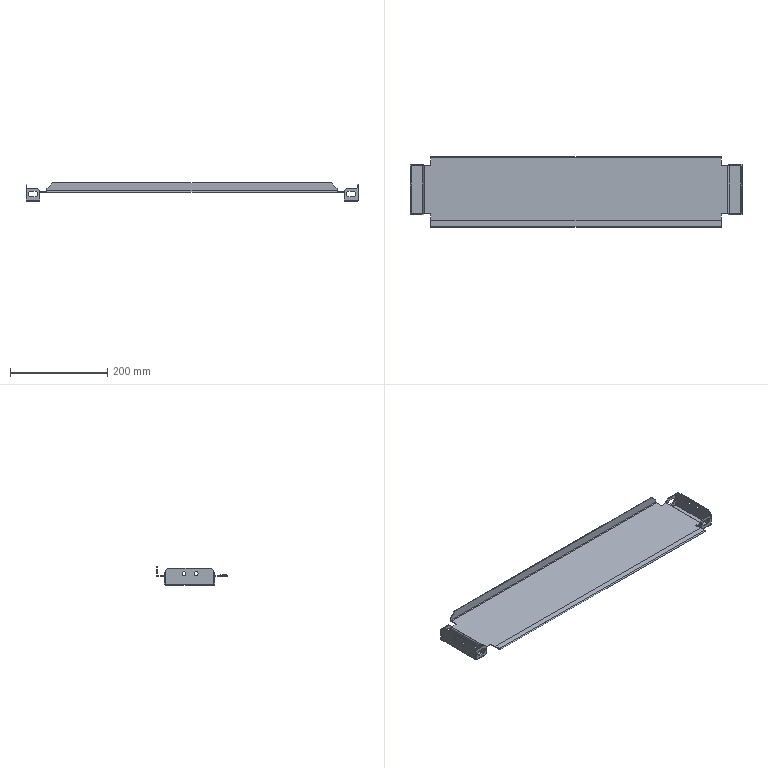Part | STEP file | 8XS320010-1~2_8XS320010.2 | 1 solid | 144 faces | box 682 x 145 x 38 mm | volume 186768 mm3 | plane 88 | cylinder 40 | spline 16 | commonest cylinder face diameters 2 x11 5 x11 8 x8 12 x8 0.1 x1 3.1 x1